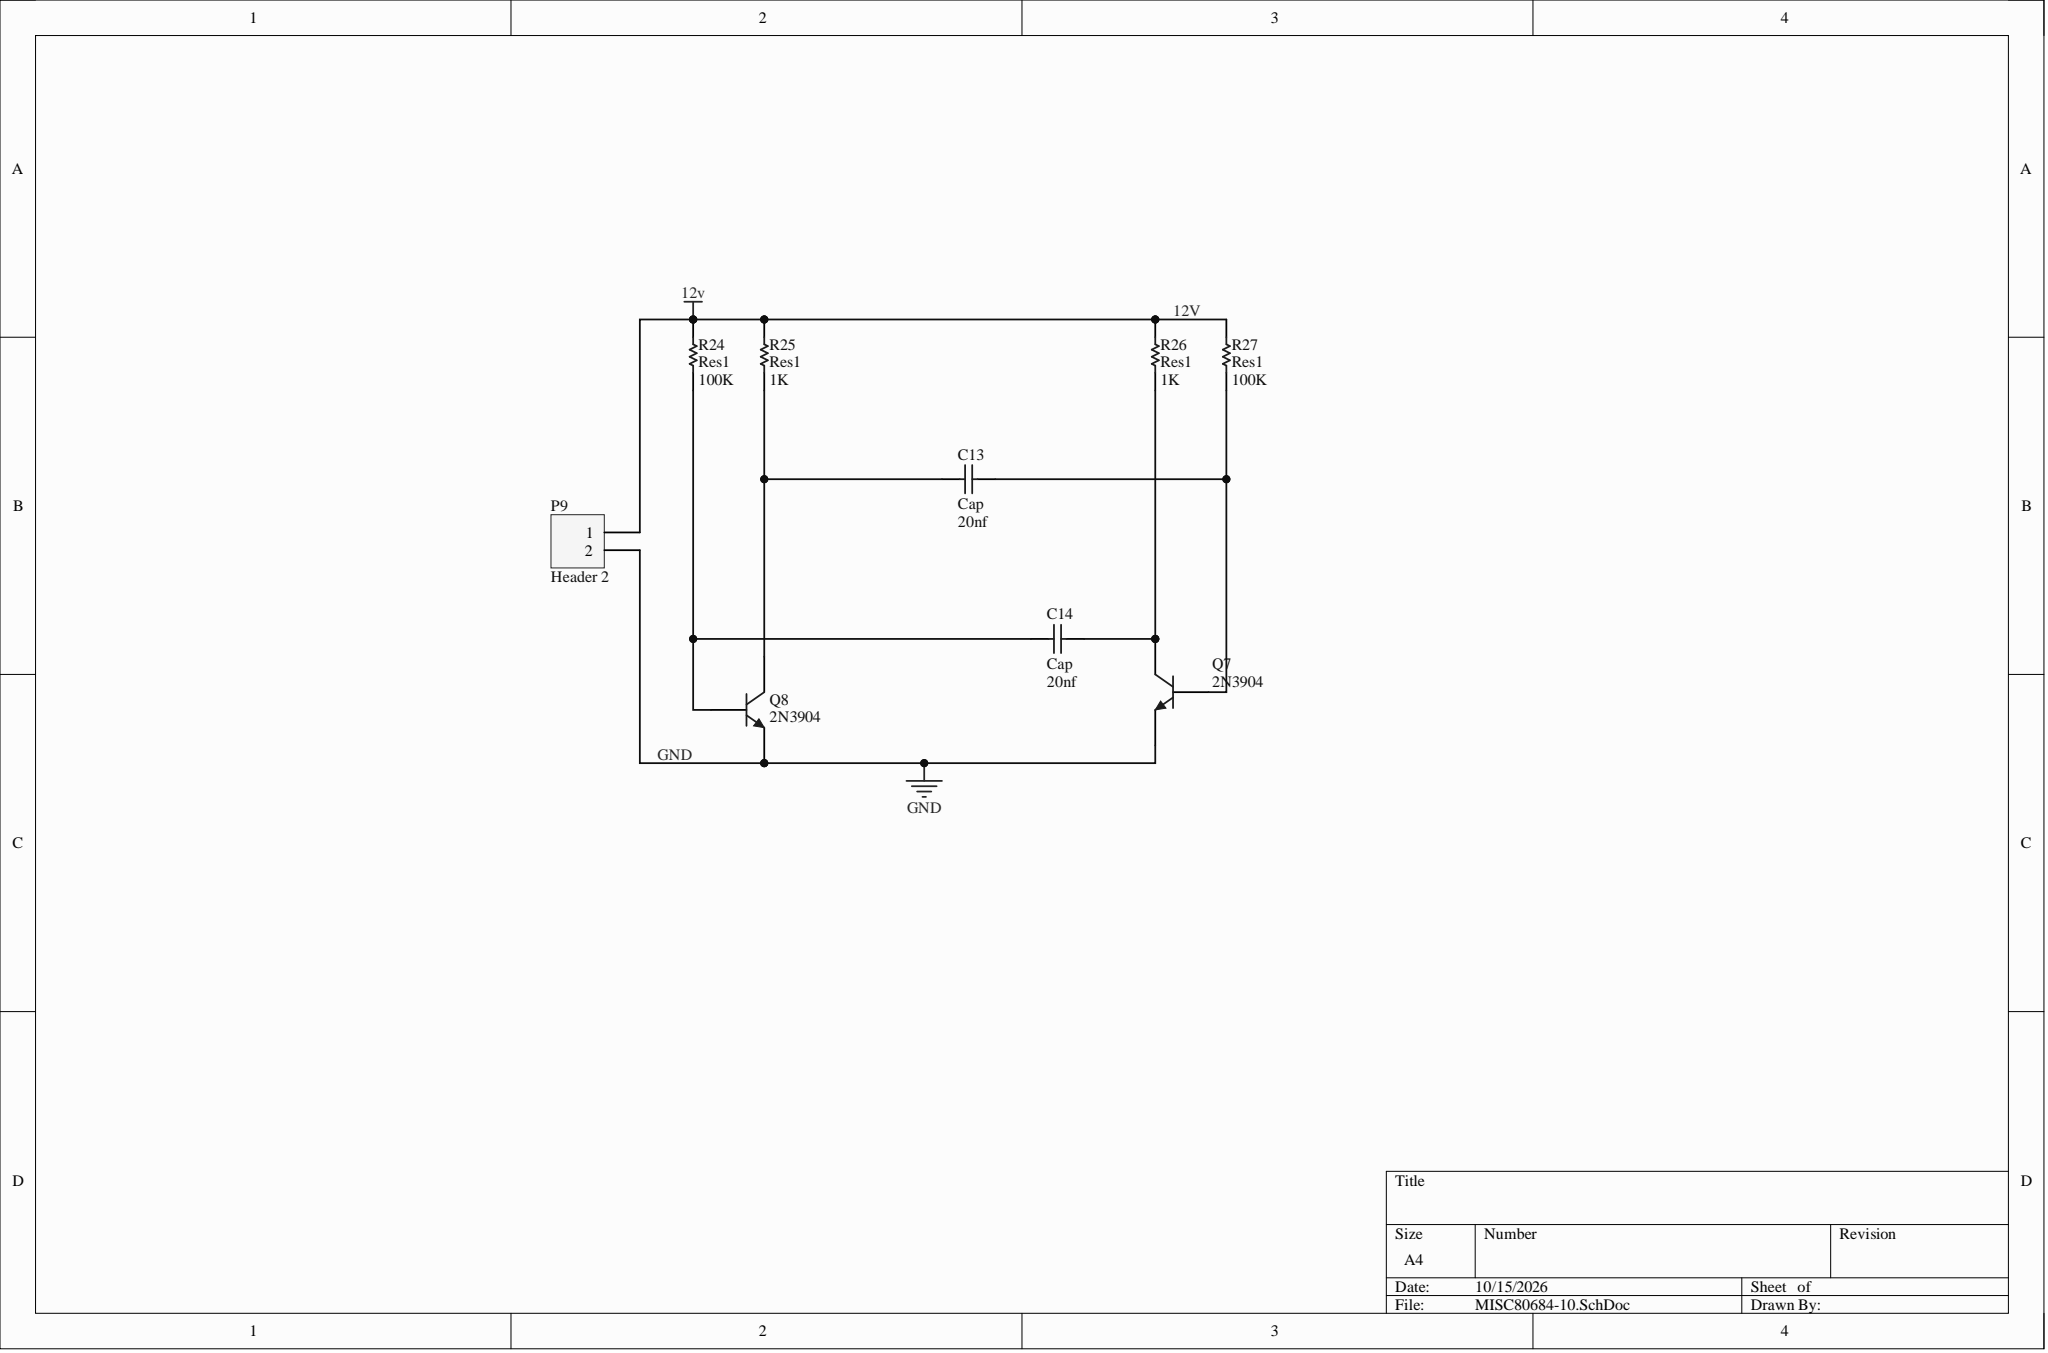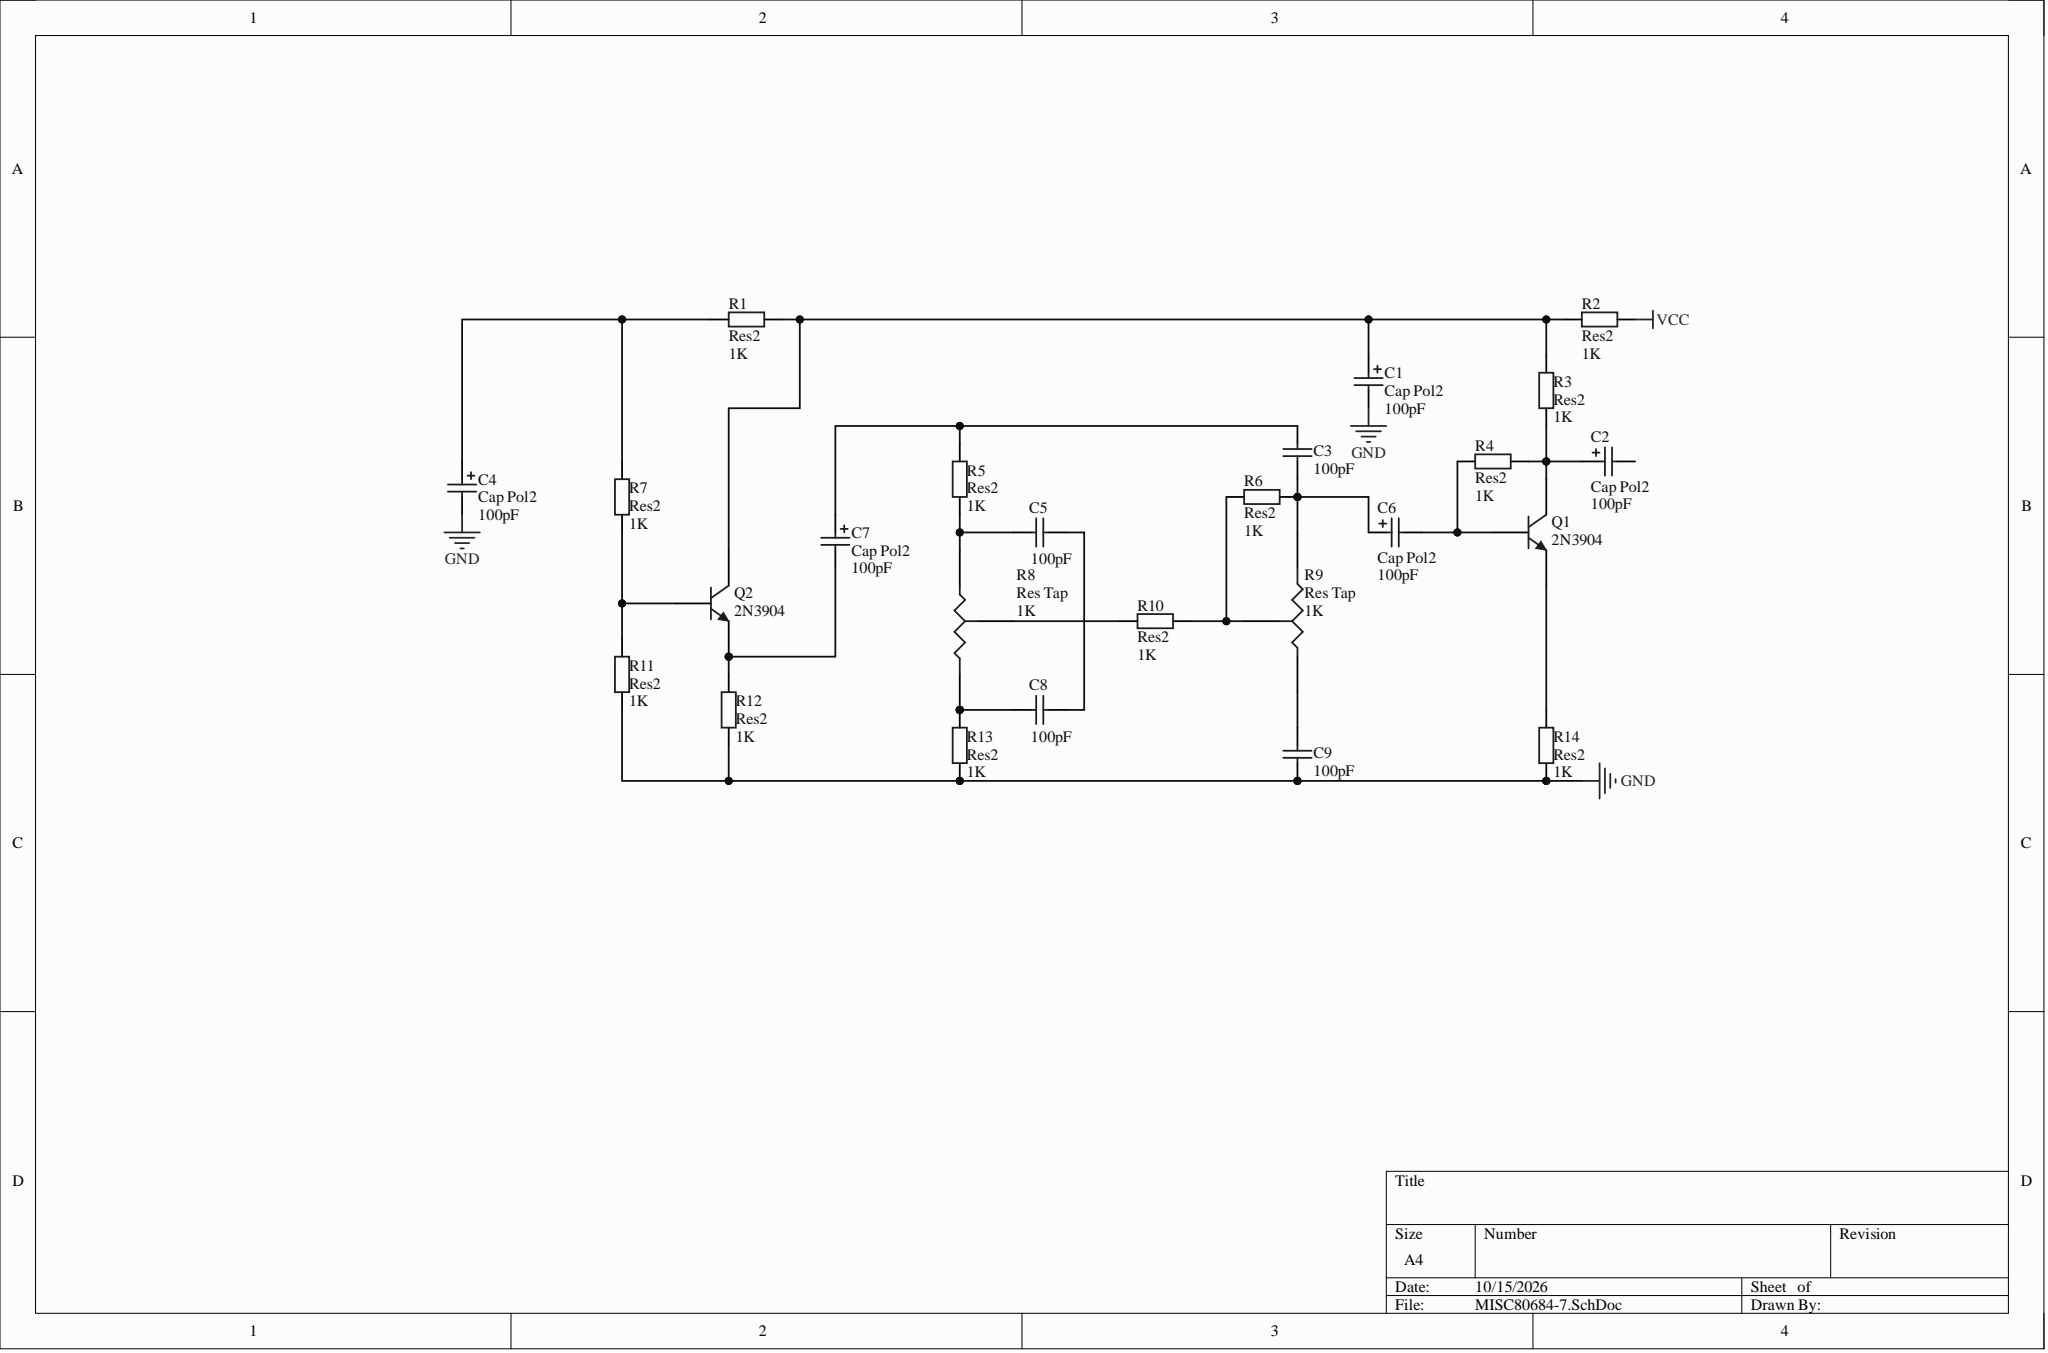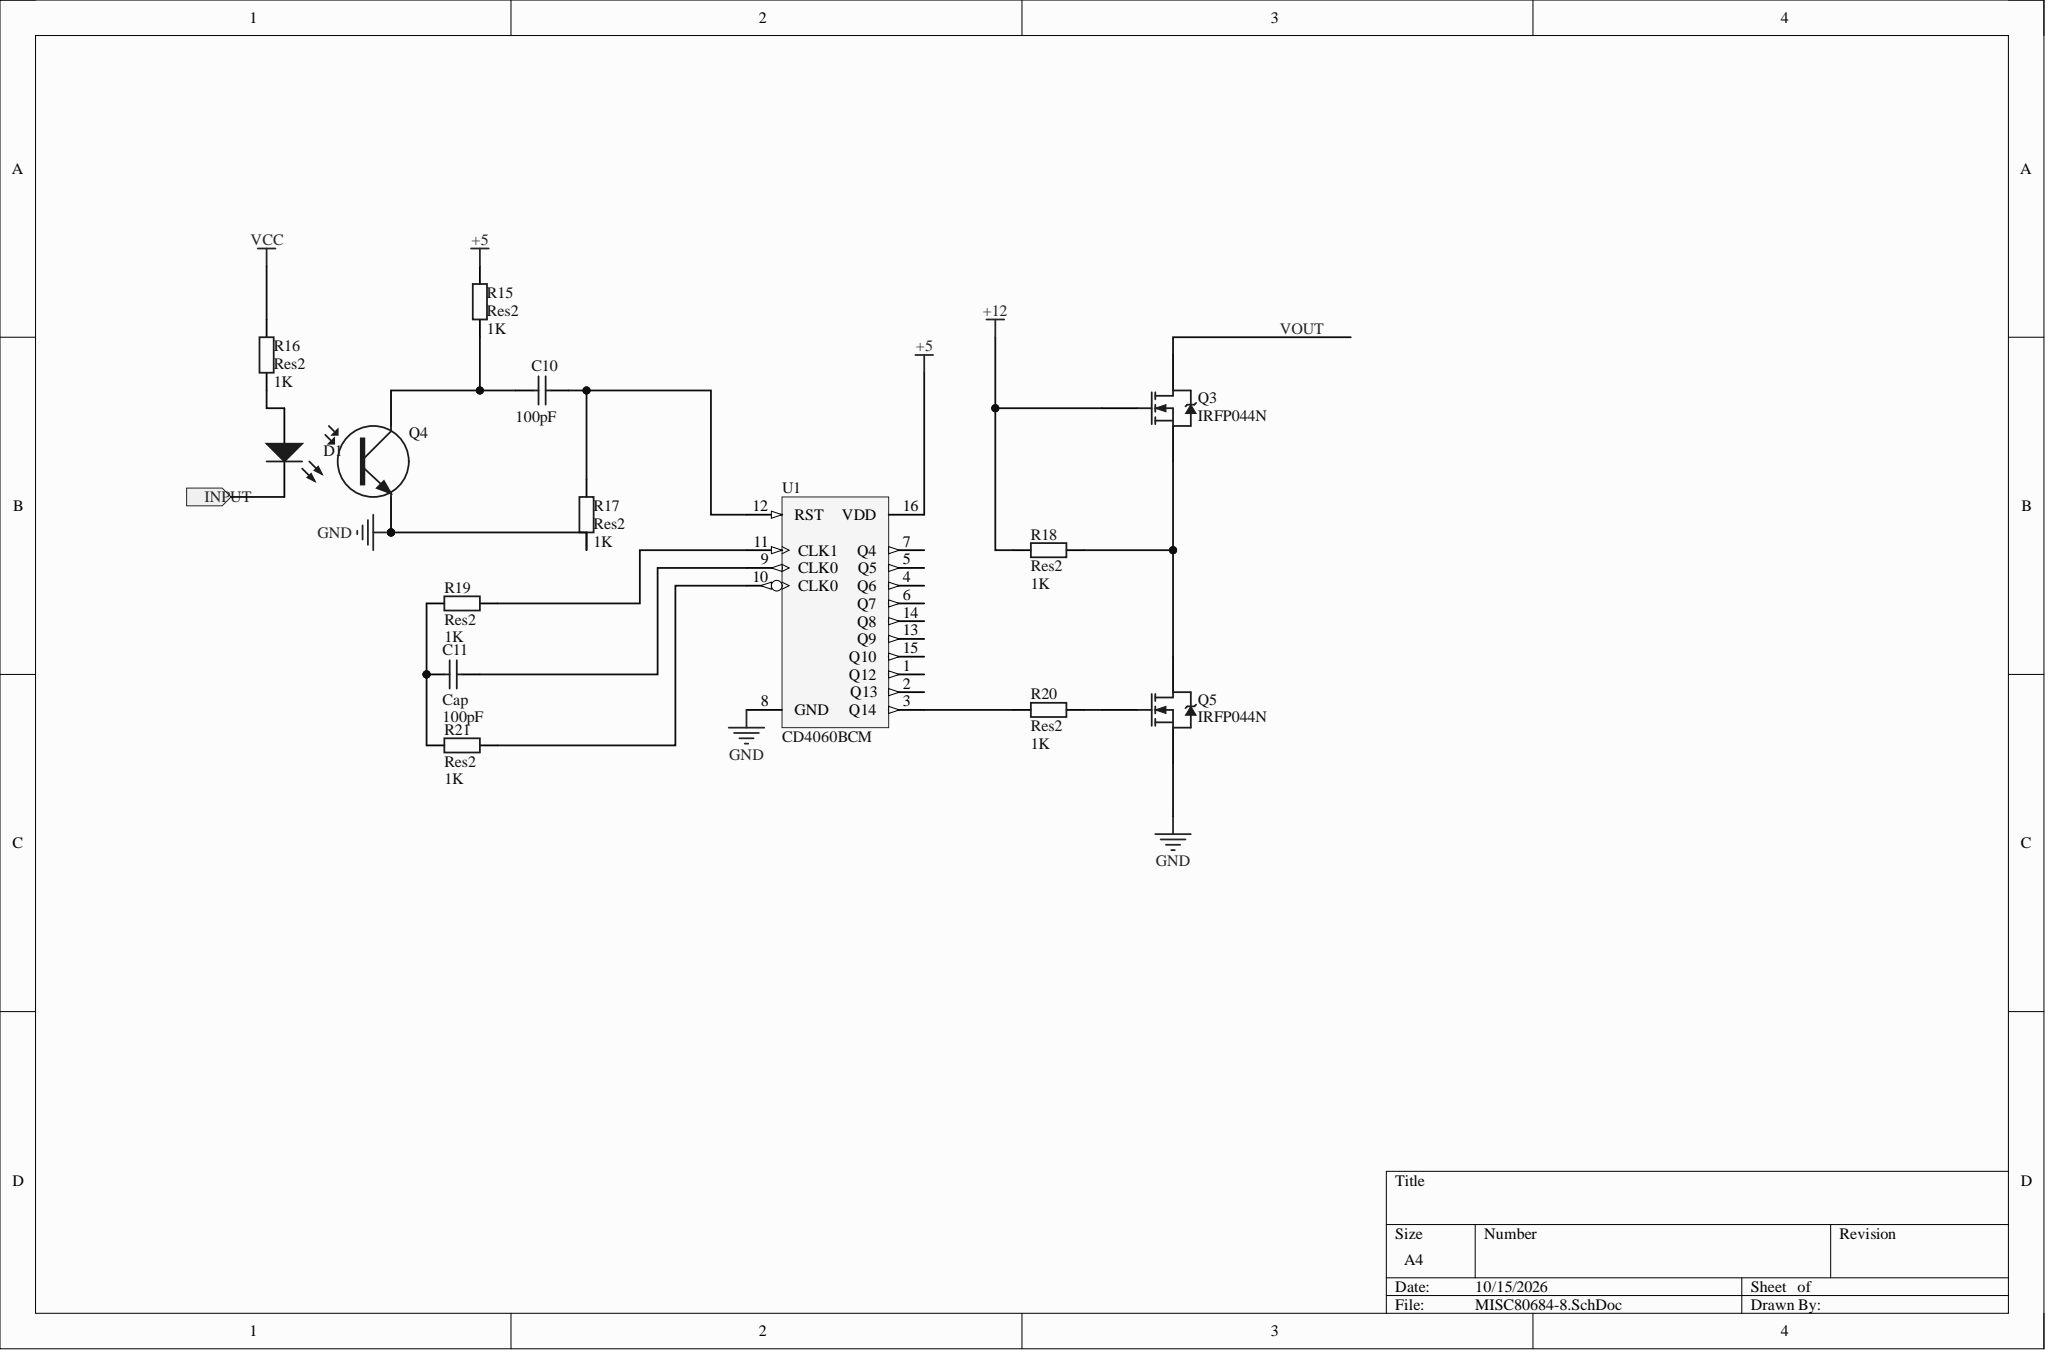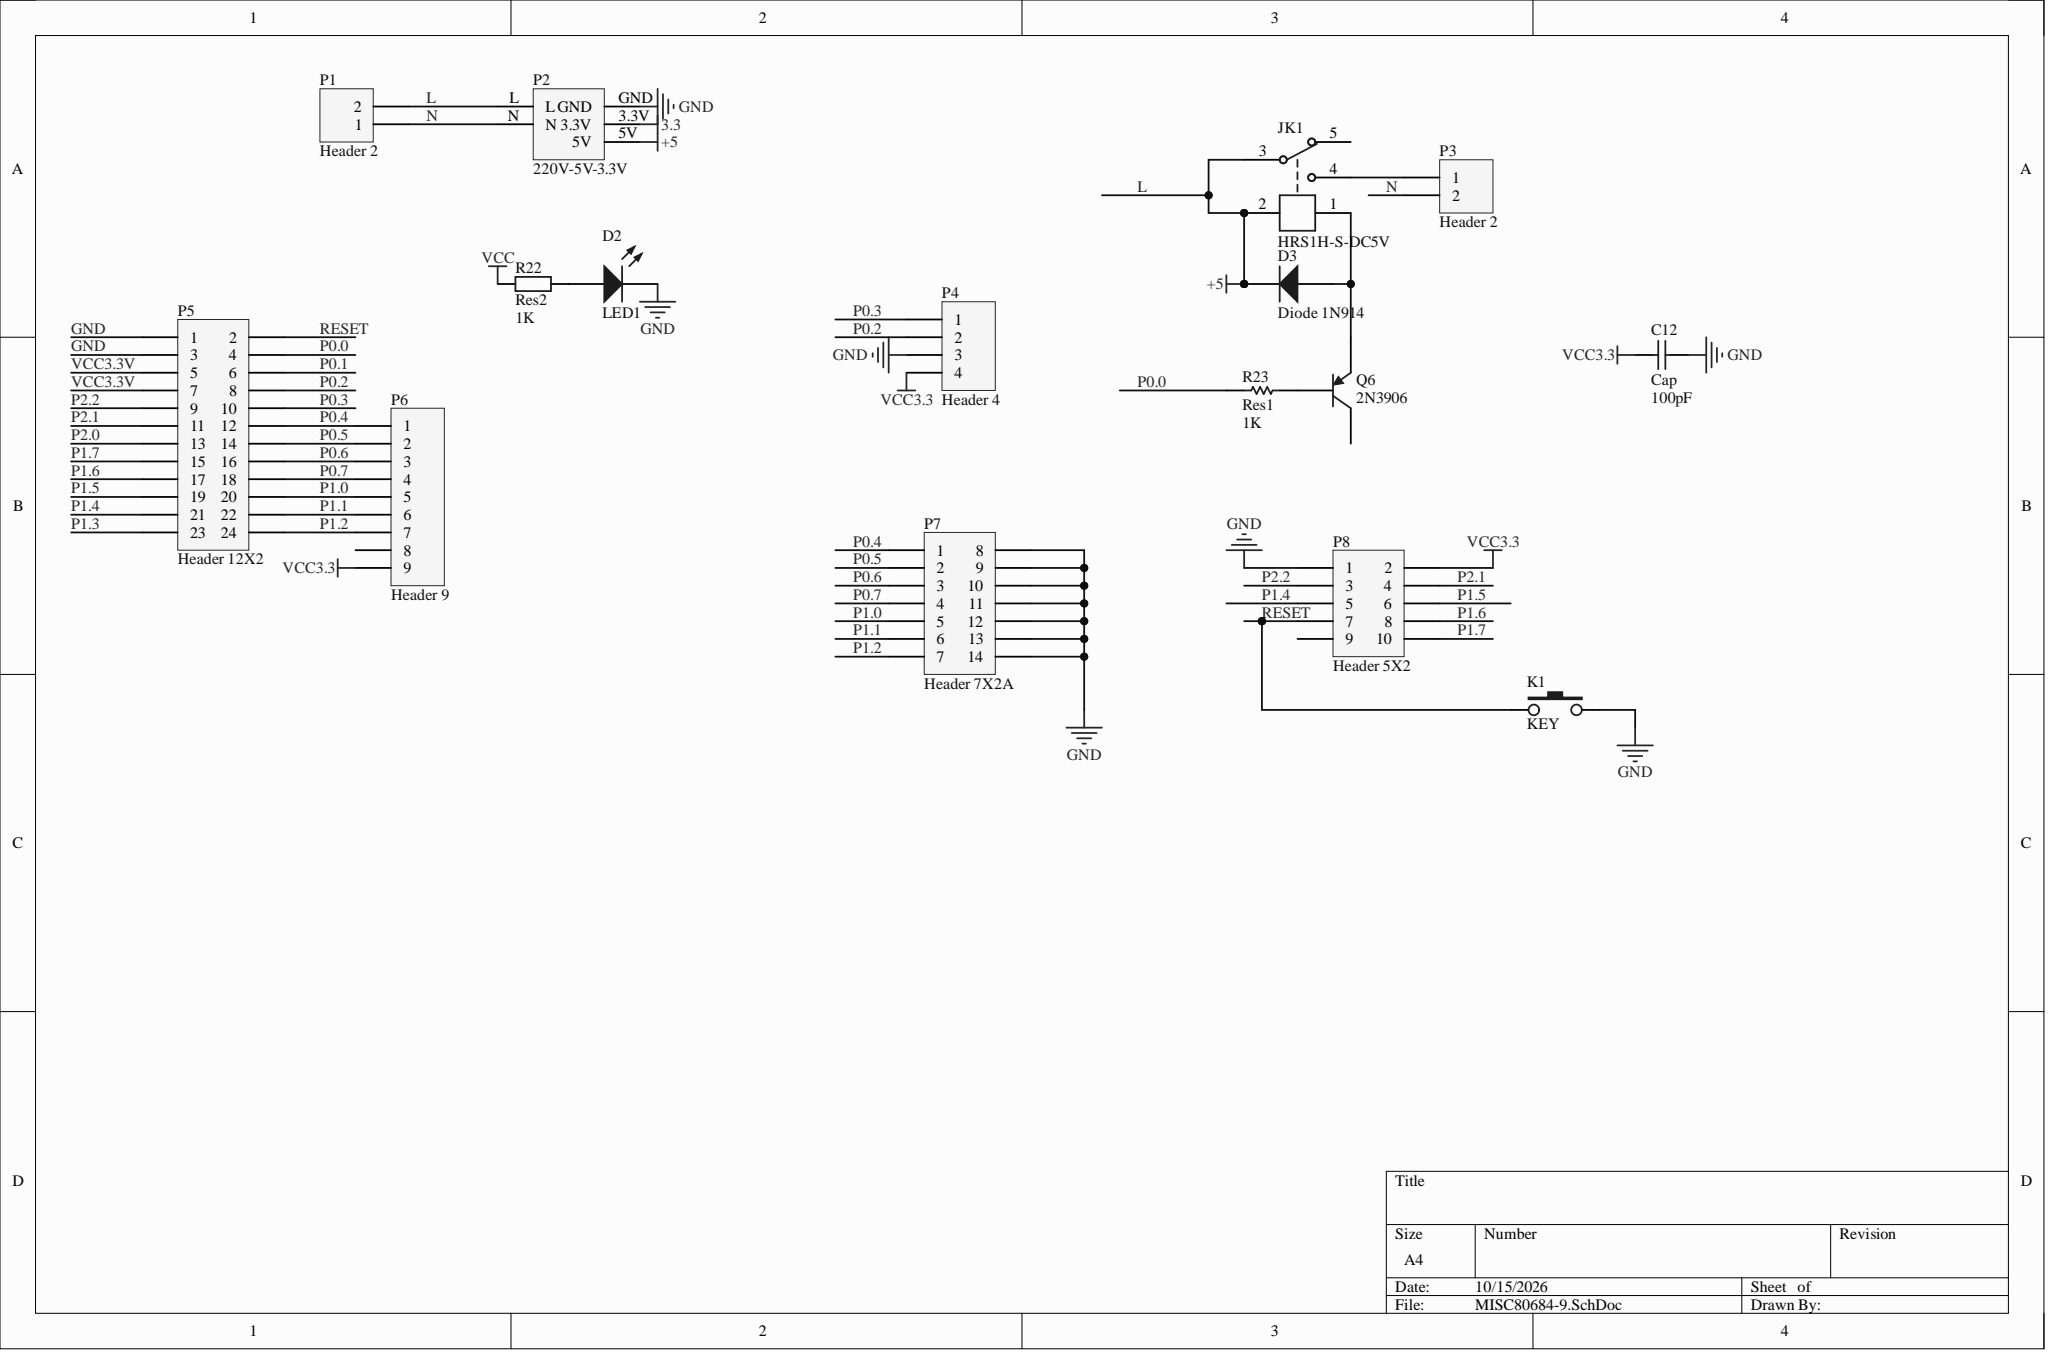Circuit board | Altium Designer | 64 parts | 58 nets
Bill of materials:
Comment,Description,Designator,Footprint,LibRef,Quantity
"Cap Pol2","Polarized Capacitor (Axial)","C1, C2, C4, C6, C7","POLAR0.8","Cap Pol2","5"
"Cap","Capacitor","C3, C5, C8, C9, C10, C11, C12, C13, C14","RAD-0.3","Cap","9"
"LED0","Typical INFRARED GaAs LED","D1","LED-0","LED0","1"
"LED1","Typical RED GaAs LED","D2","LED-1","LED1","1"
"Diode 1N914","High Conductance Fast Diode","D3","DO-35","Diode 1N914","1"
"HRS1H-S-DC5V","","JK1","HRS1H","HRS1H-S-DC5V","1"
"KEY","","K1","DIP-3X6X4.3","KEY","1"
"Header 2","Header, 2-Pin","P1, P3, P9","HDR1X2","Header 2","3"
"220V-5V-3.3V","Header, 3-Pin, Dual row","P2","HDR2X3","Header 3X2","1"
"Header 4","Header, 4-Pin","P4","HDR1X4","Header 4","1"
"Header 12X2","Header, 12-Pin, Dual row","P5","HDR2X12","Header 12X2","1"
"Header 9","Header, 9-Pin","P6","HDR1X9","Header 9","1"
"Header 7X2A","Header, 7-Pin, Dual row","P7","HDR2X7_CEN","Header 7X2A","1"
"Header 5X2","Header, 5-Pin, Dual row","P8","HDR2X5","Header 5X2","1"
"2N3904","NPN General Purpose Amplifier","Q1, Q2, Q7, Q8","TO-92A","2N3904","4"
"IRFP044N","HEXFET Power MOSFET","Q3, Q5","TO-247AC","IRFP044N","2"
"Photo NPN","NPN Phototransistor","Q4","TO-220_A","Photo NPN","1"
"2N3906","PNP General Purpose Amplifier","Q6","TO-92A","2N3906","1"
"Res2","Resistor","R1, R2, R3, R4, R5, R6, R7, R10, R11, R12, R13, R14, R15, R16, R17, R18, R19, R20, R21, R22","AXIAL-0.4","Res2","20"
"Res Tap","Tapped Resistor","R8, R9","VR3","Res Tap","2"
"Res1","Resistor","R23, R24, R25, R26, R27","AXIAL-0.3","Res1","5"
"CD4060BCM","14-Stage Ripple Carry Binary Counter","U1","M16A_N","CD4060BCM","1"
Netlist (Protel format):
[
C1
POLAR0.8
Cap Pol2



]
[
C2
POLAR0.8
Cap Pol2



]
[
C3
RAD-0.3
Cap



]
[
C4
POLAR0.8
Cap Pol2



]
[
C5
RAD-0.3
Cap



]
[
C6
POLAR0.8
Cap Pol2



]
[
C7
POLAR0.8
Cap Pol2



]
[
C8
RAD-0.3
Cap



]
[
C9
RAD-0.3
Cap



]
[
C10
RAD-0.3
Cap



]
[
C11
RAD-0.3
Cap



]
[
C12
RAD-0.3
Cap



]
[
C13
RAD-0.3
Cap



]
[
C14
RAD-0.3
Cap



]
[
D1
LED-0
LED0



]
[
D2
LED-1
LED1



]
[
D3
DO-35
Diode 1N914



]
[
JK1
HRS1H
HRS1H-S-DC5V



]
[
K1
DIP-3X6X4.3
KEY



]
[
P1
HDR1X2
Header 2



]
[
P2
HDR2X3
220V-5V-3.3V



]
[
P3
HDR1X2
Header 2



]
[
P4
HDR1X4
Header 4



]
[
P5
HDR2X12
Header 12X2



]
[
P6
HDR1X9
Header 9



]
[
P7
HDR2X7_CEN
Header 7X2A



]
[
P8
HDR2X5
Header 5X2



]
[
P9
HDR1X2
Header 2



]
[
Q1
TO-92A
2N3904



]
[
Q2
TO-92A
2N3904



]
[
Q3
TO-247AC
IRFP044N



]
[
Q4
TO-220_A
Photo NPN



]
[
Q5
TO-247AC
IRFP044N



]
[
Q6
TO-92A
2N3906



]
[
Q7
TO-92A
2N3904



]
[
Q8
TO-92A
2N3904



]
[
R1
AXIAL-0.4
Res2



]
[
R2
AXIAL-0.4
Res2



]
[
R3
AXIAL-0.4
Res2



]
[
R4
AXIAL-0.4
Res2



]
[
R5
AXIAL-0.4
Res2



]
[
R6
AXIAL-0.4
Res2



]
[
R7
AXIAL-0.4
Res2



]
[
R8
VR3
Res Tap



]
[
R9
VR3
Res Tap



]
[
R10
AXIAL-0.4
Res2



]
[
R11
AXIAL-0.4
Res2



]
[
R12
AXIAL-0.4
Res2



]
[
R13
AXIAL-0.4
Res2



]
[
R14
AXIAL-0.4
Res2



]
[
R15
AXIAL-0.4
Res2



]
[
R16
AXIAL-0.4
Res2



]
[
R17
AXIAL-0.4
Res2



]
[
R18
AXIAL-0.4
Res2



]
[
R19
AXIAL-0.4
Res2



]
[
R20
AXIAL-0.4
Res2



]
[
R21
AXIAL-0.4
Res2



]
[
R22
AXIAL-0.4
Res2



]
[
R23
AXIAL-0.3
Res1



]
[
R24
AXIAL-0.3
Res1



]
[
R25
AXIAL-0.3
Res1



]
[
R26
AXIAL-0.3
Res1



]
[
R27
AXIAL-0.3
Res1



]
[
U1
M16A_N
CD4060BCM



]
(
VCC3.3V
P5-5
P5-7
)
(
VCC3.3
C12-1
P4-4
P6-9
P8-2
)
(
VCC
R2-2
R16-1
R22-1
)
(
RESET
K1-1
P5-2
P8-7
)
(
P2.2
P5-9
P8-3
)
(
P2.1
P5-11
P8-4
)
(
P1.7
P5-15
P8-10
)
(
P1.6
P5-17
P8-8
)
(
P1.5
P5-19
P8-6
)
(
P1.4
P5-21
P8-5
)
(
P1.2
P5-24
P6-7
P7-7
)
(
P1.1
P5-22
P6-6
P7-6
)
(
P1.0
P5-20
P6-5
P7-5
)
(
P0.7
P5-18
P6-4
P7-4
)
(
P0.6
P5-16
P6-3
P7-3
)
(
P0.5
P5-14
P6-2
P7-2
)
(
P0.4
P5-12
P6-1
P7-1
)
(
P0.3
P4-1
P5-10
)
(
P0.2
P4-2
P5-8
)
(
P0.0
P5-4
R23-1
)
(
NetR21_1
R21-1
U1-10
)
(
NetR20_2
R20-2
U1-3
)
(
NetR19_1
R19-1
U1-11
)
(
NetR8_3
R8-3
R10-2
)
(
NetR6_2
R6-2
R9-3
R10-1
)
(
NetQ6_2
Q6-2
R23-2
)
(
NetQ5_1
Q5-1
R20-1
)
(
NetQ3_3
Q3-3
Q5-2
R18-1
)
(
NetQ2_2
Q2-2
R7-1
R11-2
)
(
NetQ1_1
Q1-1
R14-2
)
(
NetJK1_4
JK1-4
P3-1
)
(
NetD3_1
D3-1
JK1-1
Q6-1
)
(
NetD2_1
D2-1
R22-2
)
(
NetD1_1
D1-1
R16-2
)
(
NetC14_2
C14-2
Q7-3
R26-1
)
(
NetC14_1
C14-1
Q8-2
R24-1
)
(
NetC13_2
C13-2
Q7-2
R27-1
)
(
NetC13_1
C13-1
Q8-3
R25-1
)
(
NetC11_2
C11-2
U1-9
)
(
NetC11_1
C11-1
R19-2
R21-2
)
(
NetC10_2
C10-2
R17-2
U1-12
)
(
NetC10_1
C10-1
Q4-1
R15-2
)
(
NetC9_2
C9-2
R9-1
)
(
NetC8_1
C8-1
R8-2
R13-2
)
(
NetC7_2
C7-2
Q2-1
R12-2
)
(
NetC6_2
C6-2
Q1-2
R4-2
)
(
NetC5_2
C5-2
C8-2
)
(
NetC5_1
C5-1
R5-1
R8-1
)
(
NetC4_1
C4-1
R1-2
R7-2
)
(
NetC3_2
C3-2
C7-1
R5-2
)
(
NetC3_1
C3-1
C6-1
R6-1
R9-2
)
(
NetC2_1
C2-1
Q1-3
R3-2
R4-1
)
(
NetC1_1
C1-1
Q2-3
R1-1
R2-1
R3-1
)
(
N
P1-1
P2-N
P3-2
)
(
L
D3-2
JK1-2
JK1-3
P1-2
P2-5V
P2-L
R15-1
U1-16
)
(
GND
C1-2
C4-2
C9-1
C12-2
D2-2
K1-3
P2-GND
P4-3
P5-1
P5-3
P7-8
P7-9
P7-10
P7-11
P7-12
P7-13
P7-14
P8-1
P9-2
Q4-3
Q5-3
Q7-1
Q8-1
R11-1
R12-1
R13-1
R14-1
R17-1
U1-8
)
(
+12
Q3-1
R18-2
)
(
12V
P9-1
R24-2
R25-2
R26-2
R27-2
)